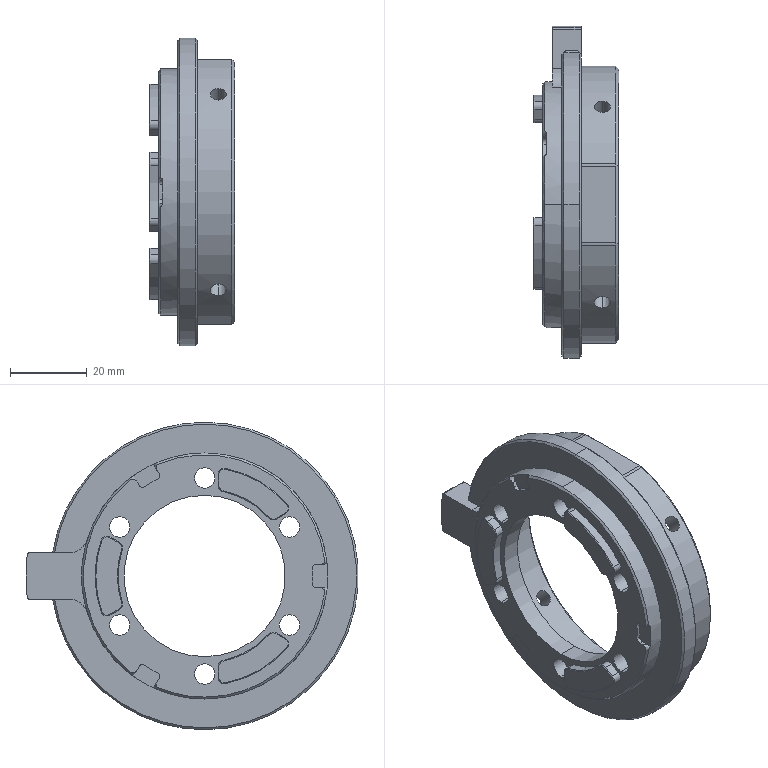Part | 1 solid | 159 faces | box 22.3 x 86.5 x 80 mm | volume 29741 mm3 | cylinder 80 | plane 36 | cone 35 | spline 6 | torus 2 | commonest cylinder face diameters 3.2 x15 5.3 x12 10 x9 4.2 x8 2 x7 1 x4